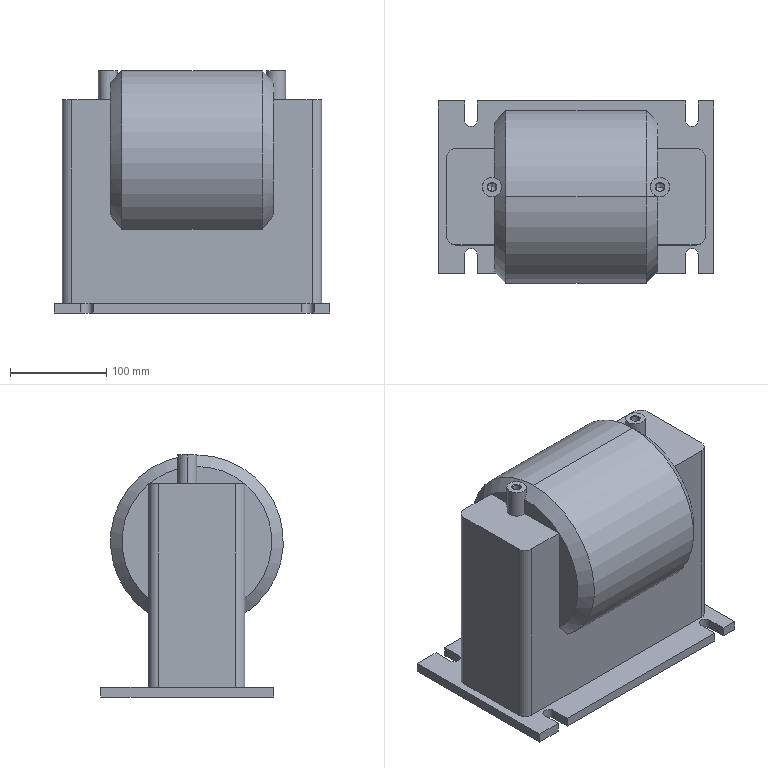Part | STEP file | 921272141 | 1 solid | 63 faces | box 287 x 190 x 252 mm | volume 8017788 mm3 | plane 34 | cylinder 18 | cone 11 | commonest cylinder face diameters 20 x8 8.5 x4 13 x4 180 x2